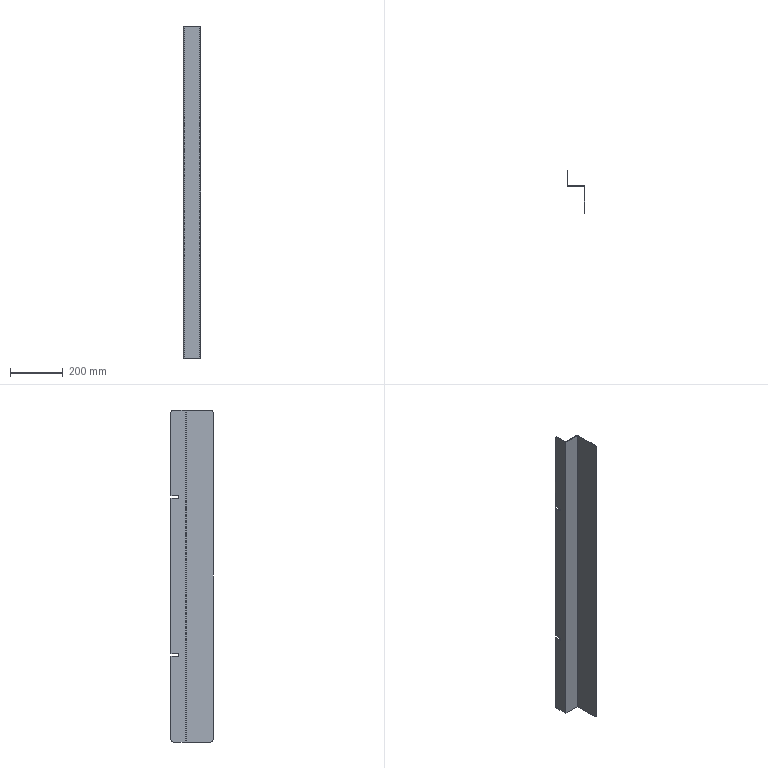Part | SolidWorks | features BaseBody 1 | 1 solid | 26 faces | box 65 x 160 x 1260 mm | volume 419104 mm3 | plane 16 | cylinder 10 | commonest cylinder face diameters 20 x4 1.473 x2 4.473 x2 9 x2
STEP:
#1=CARTESIAN_POINT('',(63.5,-103.5,10.));
#2=VERTEX_POINT('',#1);
#3=CARTESIAN_POINT('',(63.5,-93.5,0.));
#4=VERTEX_POINT('',#3);
#5=CARTESIAN_POINT('',(63.5,-93.5,10.));
#6=DIRECTION('',(1.,0.,0.));
#7=DIRECTION('',(0.,0.,1.));
#8=AXIS2_PLACEMENT_3D('',#5,#6,#7);
#9=CIRCLE('',#8,10.);
#10=EDGE_CURVE('',#2,#4,#9,.T.);
#11=ORIENTED_EDGE('',*,*,#10,.F.);
#12=CARTESIAN_POINT('',(63.5,-103.5,1250.));
#13=VERTEX_POINT('',#12);
#14=CARTESIAN_POINT('',(63.5,-103.5,1260.));
#15=DIRECTION('',(0.,0.,-1.));
#16=VECTOR('',#15,1000.);
#17=LINE('',#14,#16);
#18=EDGE_CURVE('',#13,#2,#17,.T.);
#19=ORIENTED_EDGE('',*,*,#18,.F.);
#20=CARTESIAN_POINT('',(63.5,-93.5,1260.));
#21=VERTEX_POINT('',#20);
#22=CARTESIAN_POINT('',(63.5,-93.5,1250.));
#23=DIRECTION('',(1.,0.,0.));
#24=DIRECTION('',(0.,0.,1.));
#25=AXIS2_PLACEMENT_3D('',#22,#23,#24);
#26=CIRCLE('',#25,10.);
#27=EDGE_CURVE('',#21,#13,#26,.T.);
#28=ORIENTED_EDGE('',*,*,#27,.F.);
#29=CARTESIAN_POINT('',(63.5,-0.7366,1260.));
#30=VERTEX_POINT('',#29);
#31=CARTESIAN_POINT('',(63.5,0.,1260.));
#32=DIRECTION('',(0.,-1.,0.));
#33=VECTOR('',#32,1000.);
#34=LINE('',#31,#33);
#35=EDGE_CURVE('',#30,#21,#34,.T.);
#36=ORIENTED_EDGE('',*,*,#35,.F.);
#37=CARTESIAN_POINT('',(63.5,-0.7366,0.));
#38=VERTEX_POINT('',#37);
#39=CARTESIAN_POINT('',(63.5,-0.7366,1260.));
#40=DIRECTION('',(0.,0.,1.));
#41=VECTOR('',#40,1000.);
#42=LINE('',#39,#41);
#43=EDGE_CURVE('',#38,#30,#42,.T.);
#44=ORIENTED_EDGE('',*,*,#43,.F.);
#45=CARTESIAN_POINT('',(63.5,0.,0.));
#46=DIRECTION('',(0.,1.,0.));
#47=VECTOR('',#46,1000.);
#48=LINE('',#45,#47);
#49=EDGE_CURVE('',#4,#38,#48,.T.);
#50=ORIENTED_EDGE('',*,*,#49,.F.);
#51=EDGE_LOOP('',(#11,#19,#28,#36,#44,#50));
#52=FACE_OUTER_BOUND('',#51,.T.);
#53=CARTESIAN_POINT('',(63.5,0.,1260.));
#54=DIRECTION('',(1.,0.,0.));
#55=DIRECTION('',(0.,1.,0.));
#56=AXIS2_PLACEMENT_3D('',#53,#54,#55);
#57=PLANE('',#56);
#58=ADVANCED_FACE('',(#52),#57,.F.);
#59=ORIENTED_EDGE('',*,*,#49,.T.);
#60=CARTESIAN_POINT('',(62.763,0.,0.));
#61=VERTEX_POINT('',#60);
#62=CARTESIAN_POINT('',(62.763,-0.7366,0.));
#63=DIRECTION('',(0.,0.,1.));
#64=DIRECTION('',(-1.,0.,0.));
#65=AXIS2_PLACEMENT_3D('',#62,#63,#64);
#66=CIRCLE('',#65,0.7366);
#67=EDGE_CURVE('',#38,#61,#66,.T.);
#68=ORIENTED_EDGE('',*,*,#67,.T.);
#69=CARTESIAN_POINT('',(2.237,0.,0.));
#70=VERTEX_POINT('',#69);
#71=CARTESIAN_POINT('',(0.,0.,0.));
#72=DIRECTION('',(-1.,0.,0.));
#73=VECTOR('',#72,1000.);
#74=LINE('',#71,#73);
#75=EDGE_CURVE('',#61,#70,#74,.T.);
#76=ORIENTED_EDGE('',*,*,#75,.T.);
#77=CARTESIAN_POINT('',(0.,2.237,0.));
#78=VERTEX_POINT('',#77);
#79=CARTESIAN_POINT('',(2.237,2.237,0.));
#80=DIRECTION('',(0.,0.,1.));
#81=DIRECTION('',(-1.,0.,0.));
#82=AXIS2_PLACEMENT_3D('',#79,#80,#81);
#83=CIRCLE('',#82,2.237);
#84=EDGE_CURVE('',#78,#70,#83,.T.);
#85=ORIENTED_EDGE('',*,*,#84,.F.);
#86=CARTESIAN_POINT('',(0.,46.5,0.));
#87=VERTEX_POINT('',#86);
#88=CARTESIAN_POINT('',(0.,56.5,0.));
#89=DIRECTION('',(0.,1.,0.));
#90=VECTOR('',#89,1000.);
#91=LINE('',#88,#90);
#92=EDGE_CURVE('',#78,#87,#91,.T.);
#93=ORIENTED_EDGE('',*,*,#92,.T.);
#94=CARTESIAN_POINT('',(1.5,46.5,0.));
#95=VERTEX_POINT('',#94);
#96=CARTESIAN_POINT('',(62.763,46.5,0.));
#97=DIRECTION('',(-1.,0.,0.));
#98=VECTOR('',#97,1000.);
#99=LINE('',#96,#98);
#100=EDGE_CURVE('',#95,#87,#99,.T.);
#101=ORIENTED_EDGE('',*,*,#100,.F.);
#102=CARTESIAN_POINT('',(1.5,2.237,0.));
#103=VERTEX_POINT('',#102);
#104=CARTESIAN_POINT('',(1.5,-0.7366,0.));
#105=DIRECTION('',(0.,1.,0.));
#106=VECTOR('',#105,1000.);
#107=LINE('',#104,#106);
#108=EDGE_CURVE('',#103,#95,#107,.T.);
#109=ORIENTED_EDGE('',*,*,#108,.F.);
#110=CARTESIAN_POINT('',(2.237,1.5,0.));
#111=VERTEX_POINT('',#110);
#112=CARTESIAN_POINT('',(2.237,2.237,0.));
#113=DIRECTION('',(0.,0.,1.));
#114=DIRECTION('',(-1.,0.,0.));
#115=AXIS2_PLACEMENT_3D('',#112,#113,#114);
#116=CIRCLE('',#115,0.7366);
#117=EDGE_CURVE('',#103,#111,#116,.T.);
#118=ORIENTED_EDGE('',*,*,#117,.T.);
#119=CARTESIAN_POINT('',(62.763,1.5,0.));
#120=VERTEX_POINT('',#119);
#121=CARTESIAN_POINT('',(1.5,1.5,0.));
#122=DIRECTION('',(1.,0.,0.));
#123=VECTOR('',#122,1000.);
#124=LINE('',#121,#123);
#125=EDGE_CURVE('',#111,#120,#124,.T.);
#126=ORIENTED_EDGE('',*,*,#125,.T.);
#127=CARTESIAN_POINT('',(65.,-0.7366,0.));
#128=VERTEX_POINT('',#127);
#129=CARTESIAN_POINT('',(62.763,-0.7366,0.));
#130=DIRECTION('',(0.,0.,1.));
#131=DIRECTION('',(-1.,0.,0.));
#132=AXIS2_PLACEMENT_3D('',#129,#130,#131);
#133=CIRCLE('',#132,2.237);
#134=EDGE_CURVE('',#128,#120,#133,.T.);
#135=ORIENTED_EDGE('',*,*,#134,.F.);
#136=CARTESIAN_POINT('',(65.,-93.5,0.));
#137=VERTEX_POINT('',#136);
#138=CARTESIAN_POINT('',(65.,1.5,0.));
#139=DIRECTION('',(0.,-1.,0.));
#140=VECTOR('',#139,1000.);
#141=LINE('',#138,#140);
#142=EDGE_CURVE('',#128,#137,#141,.T.);
#143=ORIENTED_EDGE('',*,*,#142,.T.);
#144=CARTESIAN_POINT('',(62.763,-93.5,0.));
#145=DIRECTION('',(-1.,0.,0.));
#146=VECTOR('',#145,1000.);
#147=LINE('',#144,#146);
#148=EDGE_CURVE('',#137,#4,#147,.T.);
#149=ORIENTED_EDGE('',*,*,#148,.T.);
#150=EDGE_LOOP('',(#59,#68,#76,#85,#93,#101,#109,#118,#126,#135,#143,#149));
#151=FACE_OUTER_BOUND('',#150,.T.);
#152=CARTESIAN_POINT('',(62.763,1.5,0.));
#153=DIRECTION('',(0.,0.,-1.));
#154=DIRECTION('',(-1.,0.,0.));
#155=AXIS2_PLACEMENT_3D('',#152,#153,#154);
#156=PLANE('',#155);
#157=ADVANCED_FACE('',(#151),#156,.T.);
#158=ORIENTED_EDGE('',*,*,#10,.T.);
#159=ORIENTED_EDGE('',*,*,#148,.F.);
#160=CARTESIAN_POINT('',(65.,-103.5,10.));
#161=VERTEX_POINT('',#160);
#162=CARTESIAN_POINT('',(65.,-93.5,10.));
#163=DIRECTION('',(-1.,0.,0.));
#164=DIRECTION('',(0.,0.,1.));
#165=AXIS2_PLACEMENT_3D('',#162,#163,#164);
#166=CIRCLE('',#165,10.);
#167=EDGE_CURVE('',#137,#161,#166,.T.);
#168=ORIENTED_EDGE('',*,*,#167,.T.);
#169=CARTESIAN_POINT('',(62.763,-103.5,10.));
#170=DIRECTION('',(-1.,0.,0.));
#171=VECTOR('',#170,1000.);
#172=LINE('',#169,#171);
#173=EDGE_CURVE('',#161,#2,#172,.T.);
#174=ORIENTED_EDGE('',*,*,#173,.T.);
#175=EDGE_LOOP('',(#158,#159,#168,#174));
#176=FACE_OUTER_BOUND('',#175,.T.);
#177=CARTESIAN_POINT('',(62.763,-93.5,10.));
#178=DIRECTION('',(-1.,0.,0.));
#179=DIRECTION('',(0.,0.,1.));
#180=AXIS2_PLACEMENT_3D('',#177,#178,#179);
#181=CYLINDRICAL_SURFACE('',#180,10.);
#182=ADVANCED_FACE('',(#176),#181,.T.);
#183=CARTESIAN_POINT('',(65.,-103.5,1250.));
#184=VERTEX_POINT('',#183);
#185=CARTESIAN_POINT('',(65.,-103.5,1260.));
#186=DIRECTION('',(0.,0.,1.));
#187=VECTOR('',#186,1000.);
#188=LINE('',#185,#187);
#189=EDGE_CURVE('',#161,#184,#188,.T.);
#190=ORIENTED_EDGE('',*,*,#189,.T.);
#191=CARTESIAN_POINT('',(65.,-103.5,1250.));
#192=DIRECTION('',(-1.,0.,0.));
#193=VECTOR('',#192,1000.);
#194=LINE('',#191,#193);
#195=EDGE_CURVE('',#184,#13,#194,.T.);
#196=ORIENTED_EDGE('',*,*,#195,.T.);
#197=ORIENTED_EDGE('',*,*,#18,.T.);
#198=ORIENTED_EDGE('',*,*,#173,.F.);
#199=EDGE_LOOP('',(#190,#196,#197,#198));
#200=FACE_OUTER_BOUND('',#199,.T.);
#201=CARTESIAN_POINT('',(65.,-103.5,1260.));
#202=DIRECTION('',(0.,-1.,0.));
#203=DIRECTION('',(0.,0.,-1.));
#204=AXIS2_PLACEMENT_3D('',#201,#202,#203);
#205=PLANE('',#204);
#206=ADVANCED_FACE('',(#200),#205,.T.);
#207=ORIENTED_EDGE('',*,*,#27,.T.);
#208=ORIENTED_EDGE('',*,*,#195,.F.);
#209=CARTESIAN_POINT('',(65.,-93.5,1260.));
#210=VERTEX_POINT('',#209);
#211=CARTESIAN_POINT('',(65.,-93.5,1250.));
#212=DIRECTION('',(-1.,0.,0.));
#213=DIRECTION('',(0.,0.,1.));
#214=AXIS2_PLACEMENT_3D('',#211,#212,#213);
#215=CIRCLE('',#214,10.);
#216=EDGE_CURVE('',#184,#210,#215,.T.);
#217=ORIENTED_EDGE('',*,*,#216,.T.);
#218=CARTESIAN_POINT('',(65.,-93.5,1260.));
#219=DIRECTION('',(-1.,0.,0.));
#220=VECTOR('',#219,1000.);
#221=LINE('',#218,#220);
#222=EDGE_CURVE('',#210,#21,#221,.T.);
#223=ORIENTED_EDGE('',*,*,#222,.T.);
#224=EDGE_LOOP('',(#207,#208,#217,#223));
#225=FACE_OUTER_BOUND('',#224,.T.);
#226=CARTESIAN_POINT('',(65.,-93.5,1250.));
#227=DIRECTION('',(-1.,0.,0.));
#228=DIRECTION('',(0.,0.,1.));
#229=AXIS2_PLACEMENT_3D('',#226,#227,#228);
#230=CYLINDRICAL_SURFACE('',#229,10.);
#231=ADVANCED_FACE('',(#225),#230,.T.);
#232=CARTESIAN_POINT('',(65.,-0.7366,1260.));
#233=VERTEX_POINT('',#232);
#234=CARTESIAN_POINT('',(65.,-0.7366,1260.));
#235=DIRECTION('',(0.,1.,0.));
#236=VECTOR('',#235,1000.);
#237=LINE('',#234,#236);
#238=EDGE_CURVE('',#210,#233,#237,.T.);
#239=ORIENTED_EDGE('',*,*,#238,.T.);
#240=CARTESIAN_POINT('',(62.763,1.5,1260.));
#241=VERTEX_POINT('',#240);
#242=CARTESIAN_POINT('',(62.763,-0.7366,1260.));
#243=DIRECTION('',(0.,0.,-1.));
#244=DIRECTION('',(-1.,0.,0.));
#245=AXIS2_PLACEMENT_3D('',#242,#243,#244);
#246=CIRCLE('',#245,2.237);
#247=EDGE_CURVE('',#241,#233,#246,.T.);
#248=ORIENTED_EDGE('',*,*,#247,.F.);
#249=CARTESIAN_POINT('',(2.237,1.5,1260.));
#250=VERTEX_POINT('',#249);
#251=CARTESIAN_POINT('',(65.,1.5,1260.));
#252=DIRECTION('',(-1.,0.,0.));
#253=VECTOR('',#252,1000.);
#254=LINE('',#251,#253);
#255=EDGE_CURVE('',#241,#250,#254,.T.);
#256=ORIENTED_EDGE('',*,*,#255,.T.);
#257=CARTESIAN_POINT('',(1.5,2.237,1260.));
#258=VERTEX_POINT('',#257);
#259=CARTESIAN_POINT('',(2.237,2.237,1260.));
#260=DIRECTION('',(0.,0.,-1.));
#261=DIRECTION('',(-1.,0.,0.));
#262=AXIS2_PLACEMENT_3D('',#259,#260,#261);
#263=CIRCLE('',#262,0.7366);
#264=EDGE_CURVE('',#250,#258,#263,.T.);
#265=ORIENTED_EDGE('',*,*,#264,.T.);
#266=CARTESIAN_POINT('',(1.5,46.5,1260.));
#267=VERTEX_POINT('',#266);
#268=CARTESIAN_POINT('',(1.5,1.5,1260.));
#269=DIRECTION('',(0.,1.,0.));
#270=VECTOR('',#269,1000.);
#271=LINE('',#268,#270);
#272=EDGE_CURVE('',#258,#267,#271,.T.);
#273=ORIENTED_EDGE('',*,*,#272,.T.);
#274=CARTESIAN_POINT('',(0.,46.5,1260.));
#275=VERTEX_POINT('',#274);
#276=CARTESIAN_POINT('',(2.237,46.5,1260.));
#277=DIRECTION('',(-1.,0.,0.));
#278=VECTOR('',#277,1000.);
#279=LINE('',#276,#278);
#280=EDGE_CURVE('',#267,#275,#279,.T.);
#281=ORIENTED_EDGE('',*,*,#280,.T.);
#282=CARTESIAN_POINT('',(0.,2.237,1260.));
#283=VERTEX_POINT('',#282);
#284=CARTESIAN_POINT('',(0.,56.5,1260.));
#285=DIRECTION('',(0.,-1.,0.));
#286=VECTOR('',#285,1000.);
#287=LINE('',#284,#286);
#288=EDGE_CURVE('',#275,#283,#287,.T.);
#289=ORIENTED_EDGE('',*,*,#288,.T.);
#290=CARTESIAN_POINT('',(2.237,0.,1260.));
#291=VERTEX_POINT('',#290);
#292=CARTESIAN_POINT('',(2.237,2.237,1260.));
#293=DIRECTION('',(0.,0.,-1.));
#294=DIRECTION('',(-1.,0.,0.));
#295=AXIS2_PLACEMENT_3D('',#292,#293,#294);
#296=CIRCLE('',#295,2.237);
#297=EDGE_CURVE('',#291,#283,#296,.T.);
#298=ORIENTED_EDGE('',*,*,#297,.F.);
#299=CARTESIAN_POINT('',(62.763,0.,1260.));
#300=VERTEX_POINT('',#299);
#301=CARTESIAN_POINT('',(0.,0.,1260.));
#302=DIRECTION('',(1.,0.,0.));
#303=VECTOR('',#302,1000.);
#304=LINE('',#301,#303);
#305=EDGE_CURVE('',#291,#300,#304,.T.);
#306=ORIENTED_EDGE('',*,*,#305,.T.);
#307=CARTESIAN_POINT('',(62.763,-0.7366,1260.));
#308=DIRECTION('',(0.,0.,-1.));
#309=DIRECTION('',(-1.,0.,0.));
#310=AXIS2_PLACEMENT_3D('',#307,#308,#309);
#311=CIRCLE('',#310,0.7366);
#312=EDGE_CURVE('',#300,#30,#311,.T.);
#313=ORIENTED_EDGE('',*,*,#312,.T.);
#314=ORIENTED_EDGE('',*,*,#35,.T.);
#315=ORIENTED_EDGE('',*,*,#222,.F.);
#316=EDGE_LOOP('',(#239,#248,#256,#265,#273,#281,#289,#298,#306,#313,#314,#315));
#317=FACE_OUTER_BOUND('',#316,.T.);
#318=CARTESIAN_POINT('',(62.763,-0.7366,1260.));
#319=DIRECTION('',(0.,0.,1.));
#320=DIRECTION('',(1.,0.,0.));
#321=AXIS2_PLACEMENT_3D('',#318,#319,#320);
#322=PLANE('',#321);
#323=ADVANCED_FACE('',(#317),#322,.T.);
#324=ORIENTED_EDGE('',*,*,#43,.T.);
#325=ORIENTED_EDGE('',*,*,#312,.F.);
#326=CARTESIAN_POINT('',(62.763,0.,1260.));
#327=DIRECTION('',(0.,0.,1.));
#328=VECTOR('',#327,1000.);
#329=LINE('',#326,#328);
#330=EDGE_CURVE('',#61,#300,#329,.T.);
#331=ORIENTED_EDGE('',*,*,#330,.F.);
#332=ORIENTED_EDGE('',*,*,#67,.F.);
#333=EDGE_LOOP('',(#324,#325,#331,#332));
#334=FACE_OUTER_BOUND('',#333,.T.);
#335=CARTESIAN_POINT('',(62.763,-0.7366,1260.));
#336=DIRECTION('',(0.,0.,-1.));
#337=DIRECTION('',(-1.,0.,0.));
#338=AXIS2_PLACEMENT_3D('',#335,#336,#337);
#339=CYLINDRICAL_SURFACE('',#338,0.7366);
#340=ADVANCED_FACE('',(#334),#339,.F.);
#341=ORIENTED_EDGE('',*,*,#238,.F.);
#342=ORIENTED_EDGE('',*,*,#216,.F.);
#343=ORIENTED_EDGE('',*,*,#189,.F.);
#344=ORIENTED_EDGE('',*,*,#167,.F.);
#345=ORIENTED_EDGE('',*,*,#142,.F.);
#346=CARTESIAN_POINT('',(65.,-0.7366,1260.));
#347=DIRECTION('',(0.,0.,1.));
#348=VECTOR('',#347,1000.);
#349=LINE('',#346,#348);
#350=EDGE_CURVE('',#128,#233,#349,.T.);
#351=ORIENTED_EDGE('',*,*,#350,.T.);
#352=EDGE_LOOP('',(#341,#342,#343,#344,#345,#351));
#353=FACE_OUTER_BOUND('',#352,.T.);
#354=CARTESIAN_POINT('',(65.,0.,1260.));
#355=DIRECTION('',(1.,0.,0.));
#356=DIRECTION('',(0.,1.,0.));
#357=AXIS2_PLACEMENT_3D('',#354,#355,#356);
#358=PLANE('',#357);
#359=ADVANCED_FACE('',(#353),#358,.T.);
#360=ORIENTED_EDGE('',*,*,#330,.T.);
#361=ORIENTED_EDGE('',*,*,#305,.F.);
#362=CARTESIAN_POINT('',(2.237,0.,1260.));
#363=DIRECTION('',(0.,0.,1.));
#364=VECTOR('',#363,1000.);
#365=LINE('',#362,#364);
#366=EDGE_CURVE('',#70,#291,#365,.T.);
#367=ORIENTED_EDGE('',*,*,#366,.F.);
#368=ORIENTED_EDGE('',*,*,#75,.F.);
#369=EDGE_LOOP('',(#360,#361,#367,#368));
#370=FACE_OUTER_BOUND('',#369,.T.);
#371=CARTESIAN_POINT('',(0.,0.,1260.));
#372=DIRECTION('',(0.,1.,0.));
#373=DIRECTION('',(0.,0.,1.));
#374=AXIS2_PLACEMENT_3D('',#371,#372,#373);
#375=PLANE('',#374);
#376=ADVANCED_FACE('',(#370),#375,.F.);
#377=ORIENTED_EDGE('',*,*,#247,.T.);
#378=ORIENTED_EDGE('',*,*,#350,.F.);
#379=ORIENTED_EDGE('',*,*,#134,.T.);
#380=CARTESIAN_POINT('',(62.763,1.5,1260.));
#381=DIRECTION('',(0.,0.,1.));
#382=VECTOR('',#381,1000.);
#383=LINE('',#380,#382);
#384=EDGE_CURVE('',#120,#241,#383,.T.);
#385=ORIENTED_EDGE('',*,*,#384,.T.);
#386=EDGE_LOOP('',(#377,#378,#379,#385));
#387=FACE_OUTER_BOUND('',#386,.T.);
#388=CARTESIAN_POINT('',(62.763,-0.7366,1260.));
#389=DIRECTION('',(0.,0.,-1.));
#390=DIRECTION('',(-1.,0.,0.));
#391=AXIS2_PLACEMENT_3D('',#388,#389,#390);
#392=CYLINDRICAL_SURFACE('',#391,2.237);
#393=ADVANCED_FACE('',(#387),#392,.T.);
#394=ORIENTED_EDGE('',*,*,#297,.T.);
#395=CARTESIAN_POINT('',(0.,2.237,1260.));
#396=DIRECTION('',(0.,0.,-1.));
#397=VECTOR('',#396,1000.);
#398=LINE('',#395,#397);
#399=EDGE_CURVE('',#283,#78,#398,.T.);
#400=ORIENTED_EDGE('',*,*,#399,.T.);
#401=ORIENTED_EDGE('',*,*,#84,.T.);
#402=ORIENTED_EDGE('',*,*,#366,.T.);
#403=EDGE_LOOP('',(#394,#400,#401,#402));
#404=FACE_OUTER_BOUND('',#403,.T.);
#405=CARTESIAN_POINT('',(2.237,2.237,1260.));
#406=DIRECTION('',(0.,0.,-1.));
#407=DIRECTION('',(-1.,0.,0.));
#408=AXIS2_PLACEMENT_3D('',#405,#406,#407);
#409=CYLINDRICAL_SURFACE('',#408,2.237);
#410=ADVANCED_FACE('',(#404),#409,.T.);
#411=ORIENTED_EDGE('',*,*,#255,.F.);
#412=ORIENTED_EDGE('',*,*,#384,.F.);
#413=ORIENTED_EDGE('',*,*,#125,.F.);
#414=CARTESIAN_POINT('',(2.237,1.5,1260.));
#415=DIRECTION('',(0.,0.,1.));
#416=VECTOR('',#415,1000.);
#417=LINE('',#414,#416);
#418=EDGE_CURVE('',#111,#250,#417,.T.);
#419=ORIENTED_EDGE('',*,*,#418,.T.);
#420=EDGE_LOOP('',(#411,#412,#413,#419));
#421=FACE_OUTER_BOUND('',#420,.T.);
#422=CARTESIAN_POINT('',(0.,1.5,1260.));
#423=DIRECTION('',(0.,1.,0.));
#424=DIRECTION('',(0.,0.,1.));
#425=AXIS2_PLACEMENT_3D('',#422,#423,#424);
#426=PLANE('',#425);
#427=ADVANCED_FACE('',(#421),#426,.T.);
#428=CARTESIAN_POINT('',(0.,56.5,10.));
#429=VERTEX_POINT('',#428);
#430=CARTESIAN_POINT('',(0.,46.5,10.));
#431=DIRECTION('',(1.,0.,0.));
#432=DIRECTION('',(0.,0.,1.));
#433=AXIS2_PLACEMENT_3D('',#430,#431,#432);
#434=CIRCLE('',#433,10.);
#435=EDGE_CURVE('',#87,#429,#434,.T.);
#436=ORIENTED_EDGE('',*,*,#435,.F.);
#437=ORIENTED_EDGE('',*,*,#92,.F.);
#438=ORIENTED_EDGE('',*,*,#399,.F.);
#439=ORIENTED_EDGE('',*,*,#288,.F.);
#440=CARTESIAN_POINT('',(0.,56.5,1250.));
#441=VERTEX_POINT('',#440);
#442=CARTESIAN_POINT('',(0.,46.5,1250.));
#443=DIRECTION('',(1.,0.,0.));
#444=DIRECTION('',(0.,0.,-1.));
#445=AXIS2_PLACEMENT_3D('',#442,#443,#444);
#446=CIRCLE('',#445,10.);
#447=EDGE_CURVE('',#441,#275,#446,.T.);
#448=ORIENTED_EDGE('',*,*,#447,.F.);
#449=CARTESIAN_POINT('',(0.,56.5,934.5));
#450=VERTEX_POINT('',#449);
#451=CARTESIAN_POINT('',(0.,56.5,1260.));
#452=DIRECTION('',(0.,0.,1.));
#453=VECTOR('',#452,1000.);
#454=LINE('',#451,#453);
#455=EDGE_CURVE('',#450,#441,#454,.T.);
#456=ORIENTED_EDGE('',*,*,#455,.F.);
#457=CARTESIAN_POINT('',(0.,31.5,934.5));
#458=VERTEX_POINT('',#457);
#459=CARTESIAN_POINT('',(0.,56.5,934.5));
#460=DIRECTION('',(0.,1.,0.));
#461=VECTOR('',#460,1000.);
#462=LINE('',#459,#461);
#463=EDGE_CURVE('',#458,#450,#462,.T.);
#464=ORIENTED_EDGE('',*,*,#463,.F.);
#465=CARTESIAN_POINT('',(0.,31.5,925.5));
#466=VERTEX_POINT('',#465);
#467=CARTESIAN_POINT('',(0.,31.5,930.));
#468=DIRECTION('',(-1.,0.,0.));
#469=DIRECTION('',(0.,0.,1.));
#470=AXIS2_PLACEMENT_3D('',#467,#468,#469);
#471=CIRCLE('',#470,4.5);
#472=EDGE_CURVE('',#466,#458,#471,.T.);
#473=ORIENTED_EDGE('',*,*,#472,.F.);
#474=CARTESIAN_POINT('',(0.,56.5,925.5));
#475=VERTEX_POINT('',#474);
#476=CARTESIAN_POINT('',(0.,56.5,925.5));
#477=DIRECTION('',(0.,-1.,0.));
#478=VECTOR('',#477,1000.);
#479=LINE('',#476,#478);
#480=EDGE_CURVE('',#475,#466,#479,.T.);
#481=ORIENTED_EDGE('',*,*,#480,.F.);
#482=CARTESIAN_POINT('',(0.,56.5,334.5));
#483=VERTEX_POINT('',#482);
#484=CARTESIAN_POINT('',(0.,56.5,1260.));
#485=DIRECTION('',(0.,0.,1.));
#486=VECTOR('',#485,1000.);
#487=LINE('',#484,#486);
#488=EDGE_CURVE('',#483,#475,#487,.T.);
#489=ORIENTED_EDGE('',*,*,#488,.F.);
#490=CARTESIAN_POINT('',(0.,31.5,334.5));
#491=VERTEX_POINT('',#490);
#492=CARTESIAN_POINT('',(0.,56.5,334.5));
#493=DIRECTION('',(0.,1.,0.));
#494=VECTOR('',#493,1000.);
#495=LINE('',#492,#494);
#496=EDGE_CURVE('',#491,#483,#495,.T.);
#497=ORIENTED_EDGE('',*,*,#496,.F.);
#498=CARTESIAN_POINT('',(0.,31.5,325.5));
#499=VERTEX_POINT('',#498);
#500=CARTESIAN_POINT('',(0.,31.5,330.));
#501=DIRECTION('',(-1.,0.,0.));
#502=DIRECTION('',(0.,0.,1.));
#503=AXIS2_PLACEMENT_3D('',#500,#501,#502);
#504=CIRCLE('',#503,4.5);
#505=EDGE_CURVE('',#499,#491,#504,.T.);
#506=ORIENTED_EDGE('',*,*,#505,.F.);
#507=CARTESIAN_POINT('',(0.,56.5,325.5));
#508=VERTEX_POINT('',#507);
#509=CARTESIAN_POINT('',(0.,56.5,325.5));
#510=DIRECTION('',(0.,-1.,0.));
#511=VECTOR('',#510,1000.);
#512=LINE('',#509,#511);
#513=EDGE_CURVE('',#508,#499,#512,.T.);
#514=ORIENTED_EDGE('',*,*,#513,.F.);
#515=CARTESIAN_POINT('',(0.,56.5,1260.));
#516=DIRECTION('',(0.,0.,1.));
#517=VECTOR('',#516,1000.);
#518=LINE('',#515,#517);
#519=EDGE_CURVE('',#429,#508,#518,.T.);
#520=ORIENTED_EDGE('',*,*,#519,.F.);
#521=EDGE_LOOP('',(#436,#437,#438,#439,#448,#456,#464,#473,#481,#489,#497,#506,#514,#520));
#522=FACE_OUTER_BOUND('',#521,.T.);
#523=CARTESIAN_POINT('',(0.,56.5,1260.));
#524=DIRECTION('',(1.,0.,0.));
#525=DIRECTION('',(0.,1.,0.));
#526=AXIS2_PLACEMENT_3D('',#523,#524,#525);
#527=PLANE('',#526);
#528=ADVANCED_FACE('',(#522),#527,.F.);
#529=CARTESIAN_POINT('',(1.5,2.237,1260.));
#530=DIRECTION('',(0.,0.,-1.));
#531=VECTOR('',#530,1000.);
#532=LINE('',#529,#531);
#533=EDGE_CURVE('',#258,#103,#532,.T.);
#534=ORIENTED_EDGE('',*,*,#533,.F.);
#535=ORIENTED_EDGE('',*,*,#264,.F.);
#536=ORIENTED_EDGE('',*,*,#418,.F.);
#537=ORIENTED_EDGE('',*,*,#117,.F.);
#538=EDGE_LOOP('',(#534,#535,#536,#537));
#539=FACE_OUTER_BOUND('',#538,.T.);
#540=CARTESIAN_POINT('',(2.237,2.237,1260.));
#541=DIRECTION('',(0.,0.,-1.));
#542=DIRECTION('',(-1.,0.,0.));
#543=AXIS2_PLACEMENT_3D('',#540,#541,#542);
#544=CYLINDRICAL_SURFACE('',#543,0.7366);
#545=ADVANCED_FACE('',(#539),#544,.F.);
#546=ORIENTED_EDGE('',*,*,#519,.T.);
#547=CARTESIAN_POINT('',(1.5,56.5,325.5));
#548=VERTEX_POINT('',#547);
#549=CARTESIAN_POINT('',(0.,56.5,325.5));
#550=DIRECTION('',(1.,0.,0.));
#551=VECTOR('',#550,1000.);
#552=LINE('',#549,#551);
#553=EDGE_CURVE('',#508,#548,#552,.T.);
#554=ORIENTED_EDGE('',*,*,#553,.T.);
#555=CARTESIAN_POINT('',(1.5,56.5,10.));
#556=VERTEX_POINT('',#555);
#557=CARTESIAN_POINT('',(1.5,56.5,1260.));
#558=DIRECTION('',(0.,0.,-1.));
#559=VECTOR('',#558,1000.);
#560=LINE('',#557,#559);
#561=EDGE_CURVE('',#548,#556,#560,.T.);
#562=ORIENTED_EDGE('',*,*,#561,.T.);
#563=CARTESIAN_POINT('',(0.,56.5,10.));
#564=DIRECTION('',(-1.,0.,0.));
#565=VECTOR('',#564,1000.);
#566=LINE('',#563,#565);
#567=EDGE_CURVE('',#556,#429,#566,.T.);
#568=ORIENTED_EDGE('',*,*,#567,.T.);
#569=EDGE_LOOP('',(#546,#554,#562,#568));
#570=FACE_OUTER_BOUND('',#569,.T.);
#571=CARTESIAN_POINT('',(0.,56.5,1260.));
#572=DIRECTION('',(0.,1.,0.));
#573=DIRECTION('',(0.,0.,1.));
#574=AXIS2_PLACEMENT_3D('',#571,#572,#573);
#575=PLANE('',#574);
#576=ADVANCED_FACE('',(#570),#575,.T.);
#577=CARTESIAN_POINT('',(1.5,46.5,10.));
#578=DIRECTION('',(-1.,0.,0.));
#579=DIRECTION('',(0.,0.,1.));
#580=AXIS2_PLACEMENT_3D('',#577,#578,#579);
#581=CIRCLE('',#580,10.);
#582=EDGE_CURVE('',#556,#95,#581,.T.);
#583=ORIENTED_EDGE('',*,*,#582,.T.);
#584=ORIENTED_EDGE('',*,*,#100,.T.);
#585=ORIENTED_EDGE('',*,*,#435,.T.);
#586=ORIENTED_EDGE('',*,*,#567,.F.);
#587=EDGE_LOOP('',(#583,#584,#585,#586));
#588=FACE_OUTER_BOUND('',#587,.T.);
#589=CARTESIAN_POINT('',(62.763,46.5,10.));
#590=DIRECTION('',(-1.,0.,0.));
#591=DIRECTION('',(0.,0.,1.));
#592=AXIS2_PLACEMENT_3D('',#589,#590,#591);
#593=CYLINDRICAL_SURFACE('',#592,10.);
#594=ADVANCED_FACE('',(#588),#593,.T.);
#595=CARTESIAN_POINT('',(1.5,56.5,1250.));
#596=VERTEX_POINT('',#595);
#597=CARTESIAN_POINT('',(1.5,46.5,1250.));
#598=DIRECTION('',(-1.,0.,0.));
#599=DIRECTION('',(0.,0.,-1.));
#600=AXIS2_PLACEMENT_3D('',#597,#598,#599);
#601=CIRCLE('',#600,10.);
#602=EDGE_CURVE('',#267,#596,#601,.T.);
#603=ORIENTED_EDGE('',*,*,#602,.T.);
#604=CARTESIAN_POINT('',(0.,56.5,1250.));
#605=DIRECTION('',(-1.,0.,0.));
#606=VECTOR('',#605,1000.);
#607=LINE('',#604,#606);
#608=EDGE_CURVE('',#596,#441,#607,.T.);
#609=ORIENTED_EDGE('',*,*,#608,.T.);
#610=ORIENTED_EDGE('',*,*,#447,.T.);
#611=ORIENTED_EDGE('',*,*,#280,.F.);
#612=EDGE_LOOP('',(#603,#609,#610,#611));
#613=FACE_OUTER_BOUND('',#612,.T.);
#614=CARTESIAN_POINT('',(0.,46.5,1250.));
#615=DIRECTION('',(1.,0.,0.));
#616=DIRECTION('',(0.,0.,-1.));
#617=AXIS2_PLACEMENT_3D('',#614,#615,#616);
#618=CYLINDRICAL_SURFACE('',#617,10.);
#619=ADVANCED_FACE('',(#613),#618,.T.);
#620=CARTESIAN_POINT('',(1.5,56.5,934.5));
#621=VERTEX_POINT('',#620);
#622=CARTESIAN_POINT('',(1.5,56.5,1260.));
#623=DIRECTION('',(0.,0.,-1.));
#624=VECTOR('',#623,1000.);
#625=LINE('',#622,#624);
#626=EDGE_CURVE('',#596,#621,#625,.T.);
#627=ORIENTED_EDGE('',*,*,#626,.T.);
#628=CARTESIAN_POINT('',(0.,56.5,934.5));
#629=DIRECTION('',(-1.,0.,0.));
#630=VECTOR('',#629,1000.);
#631=LINE('',#628,#630);
#632=EDGE_CURVE('',#621,#450,#631,.T.);
#633=ORIENTED_EDGE('',*,*,#632,.T.);
#634=ORIENTED_EDGE('',*,*,#455,.T.);
#635=ORIENTED_EDGE('',*,*,#608,.F.);
#636=EDGE_LOOP('',(#627,#633,#634,#635));
#637=FACE_OUTER_BOUND('',#636,.T.);
#638=CARTESIAN_POINT('',(0.,56.5,1260.));
#639=DIRECTION('',(0.,1.,0.));
#640=DIRECTION('',(0.,0.,1.));
#641=AXIS2_PLACEMENT_3D('',#638,#639,#640);
#642=PLANE('',#641);
#643=ADVANCED_FACE('',(#637),#642,.T.);
#644=CARTESIAN_POINT('',(1.5,31.5,934.5));
#645=VERTEX_POINT('',#644);
#646=CARTESIAN_POINT('',(1.5,61.5,934.5));
#647=DIRECTION('',(0.,1.,0.));
#648=VECTOR('',#647,1000.);
#649=LINE('',#646,#648);
#650=EDGE_CURVE('',#645,#621,#649,.T.);
#651=ORIENTED_EDGE('',*,*,#650,.F.);
#652=CARTESIAN_POINT('',(10.,31.5,934.5));
#653=DIRECTION('',(1.,0.,0.));
#654=VECTOR('',#653,1000.);
#655=LINE('',#652,#654);
#656=EDGE_CURVE('',#458,#645,#655,.T.);
#657=ORIENTED_EDGE('',*,*,#656,.F.);
#658=ORIENTED_EDGE('',*,*,#463,.T.);
#659=ORIENTED_EDGE('',*,*,#632,.F.);
#660=EDGE_LOOP('',(#651,#657,#658,#659));
#661=FACE_OUTER_BOUND('',#660,.T.);
#662=CARTESIAN_POINT('',(10.,61.5,934.5));
#663=DIRECTION('',(0.,0.,1.));
#664=DIRECTION('',(1.,0.,0.));
#665=AXIS2_PLACEMENT_3D('',#662,#663,#664);
#666=PLANE('',#665);
#667=ADVANCED_FACE('',(#661),#666,.F.);
#668=CARTESIAN_POINT('',(1.5,31.5,925.5));
#669=VERTEX_POINT('',#668);
#670=CARTESIAN_POINT('',(10.,31.5,925.5));
#671=DIRECTION('',(1.,0.,0.));
#672=VECTOR('',#671,1000.);
#673=LINE('',#670,#672);
#674=EDGE_CURVE('',#466,#669,#673,.T.);
#675=ORIENTED_EDGE('',*,*,#674,.F.);
#676=ORIENTED_EDGE('',*,*,#472,.T.);
#677=ORIENTED_EDGE('',*,*,#656,.T.);
#678=CARTESIAN_POINT('',(1.5,31.5,930.));
#679=DIRECTION('',(-1.,0.,0.));
#680=DIRECTION('',(0.,0.,1.));
#681=AXIS2_PLACEMENT_3D('',#678,#679,#680);
#682=CIRCLE('',#681,4.5);
#683=EDGE_CURVE('',#669,#645,#682,.T.);
#684=ORIENTED_EDGE('',*,*,#683,.F.);
#685=EDGE_LOOP('',(#675,#676,#677,#684));
#686=FACE_OUTER_BOUND('',#685,.T.);
#687=CARTESIAN_POINT('',(10.,31.5,930.));
#688=DIRECTION('',(-1.,0.,0.));
#689=DIRECTION('',(0.,0.,1.));
#690=AXIS2_PLACEMENT_3D('',#687,#688,#689);
#691=CYLINDRICAL_SURFACE('',#690,4.5);
#692=ADVANCED_FACE('',(#686),#691,.F.);
#693=ORIENTED_EDGE('',*,*,#480,.T.);
#694=ORIENTED_EDGE('',*,*,#674,.T.);
#695=CARTESIAN_POINT('',(1.5,56.5,925.5));
#696=VERTEX_POINT('',#695);
#697=CARTESIAN_POINT('',(1.5,61.5,925.5));
#698=DIRECTION('',(0.,-1.,0.));
#699=VECTOR('',#698,1000.);
#700=LINE('',#697,#699);
#701=EDGE_CURVE('',#696,#669,#700,.T.);
#702=ORIENTED_EDGE('',*,*,#701,.F.);
#703=CARTESIAN_POINT('',(10.,56.5,925.5));
#704=DIRECTION('',(1.,0.,0.));
#705=VECTOR('',#704,1000.);
#706=LINE('',#703,#705);
#707=EDGE_CURVE('',#475,#696,#706,.T.);
#708=ORIENTED_EDGE('',*,*,#707,.F.);
#709=EDGE_LOOP('',(#693,#694,#702,#708));
#710=FACE_OUTER_BOUND('',#709,.T.);
#711=CARTESIAN_POINT('',(10.,61.5,925.5));
#712=DIRECTION('',(0.,0.,-1.));
#713=DIRECTION('',(-1.,0.,0.));
#714=AXIS2_PLACEMENT_3D('',#711,#712,#713);
#715=PLANE('',#714);
#716=ADVANCED_FACE('',(#710),#715,.F.);
#717=CARTESIAN_POINT('',(1.5,56.5,334.5));
#718=VERTEX_POINT('',#717);
#719=CARTESIAN_POINT('',(0.,56.5,334.5));
#720=DIRECTION('',(-1.,0.,0.));
#721=VECTOR('',#720,1000.);
#722=LINE('',#719,#721);
#723=EDGE_CURVE('',#718,#483,#722,.T.);
#724=ORIENTED_EDGE('',*,*,#723,.T.);
#725=ORIENTED_EDGE('',*,*,#488,.T.);
#726=ORIENTED_EDGE('',*,*,#707,.T.);
#727=CARTESIAN_POINT('',(1.5,56.5,1260.));
#728=DIRECTION('',(0.,0.,-1.));
#729=VECTOR('',#728,1000.);
#730=LINE('',#727,#729);
#731=EDGE_CURVE('',#696,#718,#730,.T.);
#732=ORIENTED_EDGE('',*,*,#731,.T.);
#733=EDGE_LOOP('',(#724,#725,#726,#732));
#734=FACE_OUTER_BOUND('',#733,.T.);
#735=CARTESIAN_POINT('',(0.,56.5,1260.));
#736=DIRECTION('',(0.,1.,0.));
#737=DIRECTION('',(0.,0.,1.));
#738=AXIS2_PLACEMENT_3D('',#735,#736,#737);
#739=PLANE('',#738);
#740=ADVANCED_FACE('',(#734),#739,.T.);
#741=CARTESIAN_POINT('',(1.5,31.5,334.5));
#742=VERTEX_POINT('',#741);
#743=CARTESIAN_POINT('',(10.,31.5,334.5));
#744=DIRECTION('',(1.,0.,0.));
#745=VECTOR('',#744,1000.);
#746=LINE('',#743,#745);
#747=EDGE_CURVE('',#491,#742,#746,.T.);
#748=ORIENTED_EDGE('',*,*,#747,.F.);
#749=ORIENTED_EDGE('',*,*,#496,.T.);
#750=ORIENTED_EDGE('',*,*,#723,.F.);
#751=CARTESIAN_POINT('',(1.5,61.5,334.5));
#752=DIRECTION('',(0.,1.,0.));
#753=VECTOR('',#752,1000.);
#754=LINE('',#751,#753);
#755=EDGE_CURVE('',#742,#718,#754,.T.);
#756=ORIENTED_EDGE('',*,*,#755,.F.);
#757=EDGE_LOOP('',(#748,#749,#750,#756));
#758=FACE_OUTER_BOUND('',#757,.T.);
#759=CARTESIAN_POINT('',(10.,61.5,334.5));
#760=DIRECTION('',(0.,0.,1.));
#761=DIRECTION('',(1.,0.,0.));
#762=AXIS2_PLACEMENT_3D('',#759,#760,#761);
#763=PLANE('',#762);
#764=ADVANCED_FACE('',(#758),#763,.F.);
#765=CARTESIAN_POINT('',(1.5,31.5,325.5));
#766=VERTEX_POINT('',#765);
#767=CARTESIAN_POINT('',(10.,31.5,325.5));
#768=DIRECTION('',(1.,0.,0.));
#769=VECTOR('',#768,1000.);
#770=LINE('',#767,#769);
#771=EDGE_CURVE('',#499,#766,#770,.T.);
#772=ORIENTED_EDGE('',*,*,#771,.F.);
#773=ORIENTED_EDGE('',*,*,#505,.T.);
#774=ORIENTED_EDGE('',*,*,#747,.T.);
#775=CARTESIAN_POINT('',(1.5,31.5,330.));
#776=DIRECTION('',(-1.,0.,0.));
#777=DIRECTION('',(0.,0.,1.));
#778=AXIS2_PLACEMENT_3D('',#775,#776,#777);
#779=CIRCLE('',#778,4.5);
#780=EDGE_CURVE('',#766,#742,#779,.T.);
#781=ORIENTED_EDGE('',*,*,#780,.F.);
#782=EDGE_LOOP('',(#772,#773,#774,#781));
#783=FACE_OUTER_BOUND('',#782,.T.);
#784=CARTESIAN_POINT('',(10.,31.5,330.));
#785=DIRECTION('',(-1.,0.,0.));
#786=DIRECTION('',(0.,0.,1.));
#787=AXIS2_PLACEMENT_3D('',#784,#785,#786);
#788=CYLINDRICAL_SURFACE('',#787,4.5);
#789=ADVANCED_FACE('',(#783),#788,.F.);
#790=ORIENTED_EDGE('',*,*,#553,.F.);
#791=ORIENTED_EDGE('',*,*,#513,.T.);
#792=ORIENTED_EDGE('',*,*,#771,.T.);
#793=CARTESIAN_POINT('',(1.5,61.5,325.5));
#794=DIRECTION('',(0.,-1.,0.));
#795=VECTOR('',#794,1000.);
#796=LINE('',#793,#795);
#797=EDGE_CURVE('',#548,#766,#796,.T.);
#798=ORIENTED_EDGE('',*,*,#797,.F.);
#799=EDGE_LOOP('',(#790,#791,#792,#798));
#800=FACE_OUTER_BOUND('',#799,.T.);
#801=CARTESIAN_POINT('',(10.,61.5,325.5));
#802=DIRECTION('',(0.,0.,-1.));
#803=DIRECTION('',(-1.,0.,0.));
#804=AXIS2_PLACEMENT_3D('',#801,#802,#803);
#805=PLANE('',#804);
#806=ADVANCED_FACE('',(#800),#805,.F.);
#807=ORIENTED_EDGE('',*,*,#272,.F.);
#808=ORIENTED_EDGE('',*,*,#533,.T.);
#809=ORIENTED_EDGE('',*,*,#108,.T.);
#810=ORIENTED_EDGE('',*,*,#582,.F.);
#811=ORIENTED_EDGE('',*,*,#561,.F.);
#812=ORIENTED_EDGE('',*,*,#797,.T.);
#813=ORIENTED_EDGE('',*,*,#780,.T.);
#814=ORIENTED_EDGE('',*,*,#755,.T.);
#815=ORIENTED_EDGE('',*,*,#731,.F.);
#816=ORIENTED_EDGE('',*,*,#701,.T.);
#817=ORIENTED_EDGE('',*,*,#683,.T.);
#818=ORIENTED_EDGE('',*,*,#650,.T.);
#819=ORIENTED_EDGE('',*,*,#626,.F.);
#820=ORIENTED_EDGE('',*,*,#602,.F.);
#821=EDGE_LOOP('',(#807,#808,#809,#810,#811,#812,#813,#814,#815,#816,#817,#818,#819,#820));
#822=FACE_OUTER_BOUND('',#821,.T.);
#823=CARTESIAN_POINT('',(1.5,56.5,1260.));
#824=DIRECTION('',(1.,0.,0.));
#825=DIRECTION('',(0.,1.,0.));
#826=AXIS2_PLACEMENT_3D('',#823,#824,#825);
#827=PLANE('',#826);
#828=ADVANCED_FACE('',(#822),#827,.T.);
#829=CLOSED_SHELL('',(#58,#157,#182,#206,#231,#323,#340,#359,#376,#393,#410,#427,#528,#545,#576,#594,#619,#643,#667,#692,#716,#740,#764,#789,#806,#828));
#830=MANIFOLD_SOLID_BREP('',#829);
#831=CARTESIAN_POINT('',(0.,0.,0.));
#832=DIRECTION('',(0.,0.,1.));
#833=DIRECTION('',(1.,0.,0.));
#834=AXIS2_PLACEMENT_3D('',#831,#832,#833);
#835=(LENGTH_UNIT()NAMED_UNIT(*)SI_UNIT(.MILLI.,.METRE.));
#836=UNCERTAINTY_MEASURE_WITH_UNIT(LENGTH_MEASURE(0.00001),#835,'','');
#837=(NAMED_UNIT(*)PLANE_ANGLE_UNIT()SI_UNIT($,.RADIAN.));
#838=(NAMED_UNIT(*)SI_UNIT($,.STERADIAN.)SOLID_ANGLE_UNIT());
#839=(GEOMETRIC_REPRESENTATION_CONTEXT(3)GLOBAL_UNCERTAINTY_ASSIGNED_CONTEXT((#836))GLOBAL_UNIT_ASSIGNED_CONTEXT((#835,#837,#838))REPRESENTATION_CONTEXT('',''));
#840=ADVANCED_BREP_SHAPE_REPRESENTATION('',(#830,#834),#839);